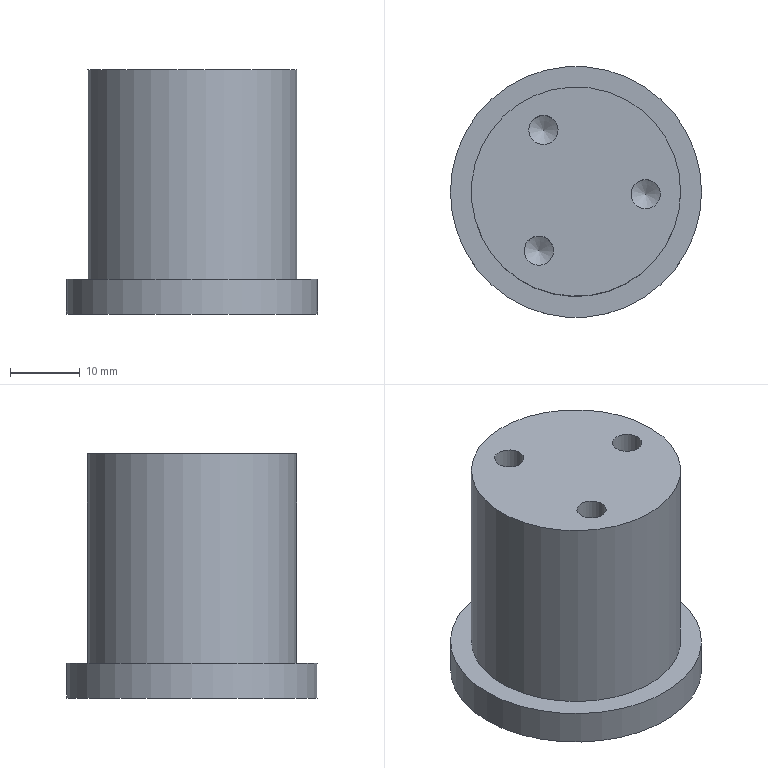Part | STEP file | 1 solid | 11 faces | box 36 x 36 x 35 mm | volume 25571 mm3 | cylinder 5 | plane 3 | cone 3 | commonest cylinder face diameters 4.2 x3 30 x1 36 x1
STEP:
#1=CARTESIAN_POINT('',(0.,0.,0.));
#2=DIRECTION('',(0.,0.,1.));
#3=DIRECTION('',(1.,0.,0.));
#4=AXIS2_PLACEMENT_3D('',#1,#2,#3);
#5=CARTESIAN_POINT('',(15.,0.,35.));
#6=VERTEX_POINT('',#5);
#7=CARTESIAN_POINT('',(0.,0.,35.));
#8=DIRECTION('',(0.,0.,-1.));
#9=DIRECTION('',(1.,0.,0.));
#10=AXIS2_PLACEMENT_3D('',#7,#8,#9);
#11=CIRCLE('',#10,15.);
#12=CARTESIAN_POINT('',(0.,0.,5.));
#13=DIRECTION('',(0.,0.,1.));
#14=DIRECTION('',(1.,0.,0.));
#15=AXIS2_PLACEMENT_3D('',#12,#13,#14);
#16=CYLINDRICAL_SURFACE('',#15,15.);
#17=CARTESIAN_POINT('',(6.283,30.));
#18=DIRECTION('',(-1.,0.));
#19=VECTOR('',#18,1.);
#20=LINE('',#17,#19);
#21=(GEOMETRIC_REPRESENTATION_CONTEXT(2)PARAMETRIC_REPRESENTATION_CONTEXT()REPRESENTATION_CONTEXT('',''));
#22=DEFINITIONAL_REPRESENTATION('',(#20),#21);
#23=PCURVE('',#16,#22);
#24=CARTESIAN_POINT('',(0.,0.,35.));
#25=DIRECTION('',(0.,0.,1.));
#26=DIRECTION('',(1.,0.,0.));
#27=AXIS2_PLACEMENT_3D('',#24,#25,#26);
#28=PLANE('',#27);
#29=CARTESIAN_POINT('',(15.,0.));
#30=CARTESIAN_POINT('',(15.,-25.981));
#31=CARTESIAN_POINT('',(-7.5,-12.99));
#32=CARTESIAN_POINT('',(-30.,0.));
#33=CARTESIAN_POINT('',(-7.5,12.99));
#34=CARTESIAN_POINT('',(15.,25.981));
#35=CARTESIAN_POINT('',(15.,0.));
#36=(BOUNDED_CURVE()B_SPLINE_CURVE(2,(#29,#30,#31,#32,#33,#34,#35),.UNSPECIFIED.,.T.,.F.)B_SPLINE_CURVE_WITH_KNOTS((1,2,2,2,2,1),(-2.094,0.,2.094,4.189,6.283,8.378),.UNSPECIFIED.)CURVE()GEOMETRIC_REPRESENTATION_ITEM()RATIONAL_B_SPLINE_CURVE((1.,0.5,1.,0.5,1.,0.5,1.))REPRESENTATION_ITEM(''));
#37=(GEOMETRIC_REPRESENTATION_CONTEXT(2)PARAMETRIC_REPRESENTATION_CONTEXT()REPRESENTATION_CONTEXT('',''));
#38=DEFINITIONAL_REPRESENTATION('',(#36),#37);
#39=PCURVE('',#28,#38);
#40=SURFACE_CURVE('',#11,(#23,#39),.PCURVE_S1.);
#41=EDGE_CURVE('',#6,#6,#40,.T.);
#42=ORIENTED_EDGE('',*,*,#41,.T.);
#43=CARTESIAN_POINT('',(15.,0.,5.));
#44=VERTEX_POINT('',#43);
#45=CARTESIAN_POINT('',(15.,0.,5.));
#46=CARTESIAN_POINT('',(15.,0.,35.));
#47=B_SPLINE_CURVE_WITH_KNOTS('',1,(#45,#46),.UNSPECIFIED.,.F.,.F.,(2,2),(0.,30.),.PIECEWISE_BEZIER_KNOTS.);
#48=CARTESIAN_POINT('',(0.,0.));
#49=DIRECTION('',(0.,1.));
#50=VECTOR('',#49,1.);
#51=LINE('',#48,#50);
#52=(GEOMETRIC_REPRESENTATION_CONTEXT(2)PARAMETRIC_REPRESENTATION_CONTEXT()REPRESENTATION_CONTEXT('',''));
#53=DEFINITIONAL_REPRESENTATION('',(#51),#52);
#54=PCURVE('',#16,#53);
#55=CARTESIAN_POINT('',(6.283,0.));
#56=DIRECTION('',(0.,1.));
#57=VECTOR('',#56,1.);
#58=LINE('',#55,#57);
#59=(GEOMETRIC_REPRESENTATION_CONTEXT(2)PARAMETRIC_REPRESENTATION_CONTEXT()REPRESENTATION_CONTEXT('',''));
#60=DEFINITIONAL_REPRESENTATION('',(#58),#59);
#61=PCURVE('',#16,#60);
#62=SEAM_CURVE('',#47,(#54,#61),.PCURVE_S1.);
#63=EDGE_CURVE('',#44,#6,#62,.T.);
#64=ORIENTED_EDGE('',*,*,#63,.F.);
#65=CARTESIAN_POINT('',(0.,0.,5.));
#66=DIRECTION('',(0.,0.,1.));
#67=DIRECTION('',(1.,0.,0.));
#68=AXIS2_PLACEMENT_3D('',#65,#66,#67);
#69=CIRCLE('',#68,15.);
#70=CARTESIAN_POINT('',(0.,0.));
#71=DIRECTION('',(1.,0.));
#72=VECTOR('',#71,1.);
#73=LINE('',#70,#72);
#74=(GEOMETRIC_REPRESENTATION_CONTEXT(2)PARAMETRIC_REPRESENTATION_CONTEXT()REPRESENTATION_CONTEXT('',''));
#75=DEFINITIONAL_REPRESENTATION('',(#73),#74);
#76=PCURVE('',#16,#75);
#77=CARTESIAN_POINT('',(0.,0.,5.));
#78=DIRECTION('',(0.,0.,1.));
#79=DIRECTION('',(1.,0.,0.));
#80=AXIS2_PLACEMENT_3D('',#77,#78,#79);
#81=PLANE('',#80);
#82=CARTESIAN_POINT('',(0.,0.));
#83=DIRECTION('',(1.,0.));
#84=AXIS2_PLACEMENT_2D('',#82,#83);
#85=CIRCLE('',#84,15.);
#86=(GEOMETRIC_REPRESENTATION_CONTEXT(2)PARAMETRIC_REPRESENTATION_CONTEXT()REPRESENTATION_CONTEXT('',''));
#87=DEFINITIONAL_REPRESENTATION('',(#85),#86);
#88=PCURVE('',#81,#87);
#89=SURFACE_CURVE('',#69,(#76,#88),.PCURVE_S1.);
#90=EDGE_CURVE('',#44,#44,#89,.T.);
#91=ORIENTED_EDGE('',*,*,#90,.T.);
#92=ORIENTED_EDGE('',*,*,#63,.T.);
#93=EDGE_LOOP('',(#42,#64,#91,#92));
#94=FACE_BOUND('',#93,.T.);
#95=ADVANCED_FACE('',(#94),#16,.T.);
#96=CARTESIAN_POINT('',(-2.577,8.839,35.));
#97=VERTEX_POINT('',#96);
#98=CARTESIAN_POINT('',(-4.677,8.839,35.));
#99=DIRECTION('',(0.,0.,-1.));
#100=DIRECTION('',(1.,0.,0.));
#101=AXIS2_PLACEMENT_3D('',#98,#99,#100);
#102=CIRCLE('',#101,2.1);
#103=CARTESIAN_POINT('',(-2.577,8.839));
#104=CARTESIAN_POINT('',(-2.577,5.201));
#105=CARTESIAN_POINT('',(-5.727,7.02));
#106=CARTESIAN_POINT('',(-8.877,8.839));
#107=CARTESIAN_POINT('',(-5.727,10.657));
#108=CARTESIAN_POINT('',(-2.577,12.476));
#109=CARTESIAN_POINT('',(-2.577,8.839));
#110=(BOUNDED_CURVE()B_SPLINE_CURVE(2,(#103,#104,#105,#106,#107,#108,#109),.UNSPECIFIED.,.T.,.F.)B_SPLINE_CURVE_WITH_KNOTS((1,2,2,2,2,1),(-2.094,0.,2.094,4.189,6.283,8.378),.UNSPECIFIED.)CURVE()GEOMETRIC_REPRESENTATION_ITEM()RATIONAL_B_SPLINE_CURVE((1.,0.5,1.,0.5,1.,0.5,1.))REPRESENTATION_ITEM(''));
#111=(GEOMETRIC_REPRESENTATION_CONTEXT(2)PARAMETRIC_REPRESENTATION_CONTEXT()REPRESENTATION_CONTEXT('',''));
#112=DEFINITIONAL_REPRESENTATION('',(#110),#111);
#113=PCURVE('',#28,#112);
#114=CARTESIAN_POINT('',(-4.677,8.839,35.));
#115=DIRECTION('',(0.,0.,1.));
#116=DIRECTION('',(1.,0.,0.));
#117=AXIS2_PLACEMENT_3D('',#114,#115,#116);
#118=CYLINDRICAL_SURFACE('',#117,2.1);
#119=CARTESIAN_POINT('',(6.283,0.));
#120=DIRECTION('',(-1.,0.));
#121=VECTOR('',#120,1.);
#122=LINE('',#119,#121);
#123=(GEOMETRIC_REPRESENTATION_CONTEXT(2)PARAMETRIC_REPRESENTATION_CONTEXT()REPRESENTATION_CONTEXT('',''));
#124=DEFINITIONAL_REPRESENTATION('',(#122),#123);
#125=PCURVE('',#118,#124);
#126=SURFACE_CURVE('',#102,(#113,#125),.PCURVE_S1.);
#127=EDGE_CURVE('',#97,#97,#126,.T.);
#128=ORIENTED_EDGE('',*,*,#127,.T.);
#129=EDGE_LOOP('',(#128));
#130=FACE_BOUND('',#129,.T.);
#131=CARTESIAN_POINT('',(-3.216,-8.47,35.));
#132=VERTEX_POINT('',#131);
#133=CARTESIAN_POINT('',(-5.316,-8.47,35.));
#134=DIRECTION('',(0.,0.,-1.));
#135=DIRECTION('',(1.,0.,0.));
#136=AXIS2_PLACEMENT_3D('',#133,#134,#135);
#137=CIRCLE('',#136,2.1);
#138=CARTESIAN_POINT('',(-3.216,-8.47));
#139=CARTESIAN_POINT('',(-3.216,-12.107));
#140=CARTESIAN_POINT('',(-6.366,-10.289));
#141=CARTESIAN_POINT('',(-9.516,-8.47));
#142=CARTESIAN_POINT('',(-6.366,-6.651));
#143=CARTESIAN_POINT('',(-3.216,-4.833));
#144=CARTESIAN_POINT('',(-3.216,-8.47));
#145=(BOUNDED_CURVE()B_SPLINE_CURVE(2,(#138,#139,#140,#141,#142,#143,#144),.UNSPECIFIED.,.T.,.F.)B_SPLINE_CURVE_WITH_KNOTS((1,2,2,2,2,1),(-2.094,0.,2.094,4.189,6.283,8.378),.UNSPECIFIED.)CURVE()GEOMETRIC_REPRESENTATION_ITEM()RATIONAL_B_SPLINE_CURVE((1.,0.5,1.,0.5,1.,0.5,1.))REPRESENTATION_ITEM(''));
#146=(GEOMETRIC_REPRESENTATION_CONTEXT(2)PARAMETRIC_REPRESENTATION_CONTEXT()REPRESENTATION_CONTEXT('',''));
#147=DEFINITIONAL_REPRESENTATION('',(#145),#146);
#148=PCURVE('',#28,#147);
#149=CARTESIAN_POINT('',(-5.316,-8.47,35.));
#150=DIRECTION('',(0.,0.,1.));
#151=DIRECTION('',(1.,0.,0.));
#152=AXIS2_PLACEMENT_3D('',#149,#150,#151);
#153=CYLINDRICAL_SURFACE('',#152,2.1);
#154=CARTESIAN_POINT('',(6.283,0.));
#155=DIRECTION('',(-1.,0.));
#156=VECTOR('',#155,1.);
#157=LINE('',#154,#156);
#158=(GEOMETRIC_REPRESENTATION_CONTEXT(2)PARAMETRIC_REPRESENTATION_CONTEXT()REPRESENTATION_CONTEXT('',''));
#159=DEFINITIONAL_REPRESENTATION('',(#157),#158);
#160=PCURVE('',#153,#159);
#161=SURFACE_CURVE('',#137,(#148,#160),.PCURVE_S1.);
#162=EDGE_CURVE('',#132,#132,#161,.T.);
#163=ORIENTED_EDGE('',*,*,#162,.T.);
#164=EDGE_LOOP('',(#163));
#165=FACE_BOUND('',#164,.T.);
#166=CARTESIAN_POINT('',(12.093,-0.3685,35.));
#167=VERTEX_POINT('',#166);
#168=CARTESIAN_POINT('',(9.993,-0.3685,35.));
#169=DIRECTION('',(0.,0.,-1.));
#170=DIRECTION('',(1.,0.,0.));
#171=AXIS2_PLACEMENT_3D('',#168,#169,#170);
#172=CIRCLE('',#171,2.1);
#173=CARTESIAN_POINT('',(12.093,-0.3685));
#174=CARTESIAN_POINT('',(12.093,-4.006));
#175=CARTESIAN_POINT('',(8.943,-2.187));
#176=CARTESIAN_POINT('',(5.793,-0.3685));
#177=CARTESIAN_POINT('',(8.943,1.45));
#178=CARTESIAN_POINT('',(12.093,3.269));
#179=CARTESIAN_POINT('',(12.093,-0.3685));
#180=(BOUNDED_CURVE()B_SPLINE_CURVE(2,(#173,#174,#175,#176,#177,#178,#179),.UNSPECIFIED.,.T.,.F.)B_SPLINE_CURVE_WITH_KNOTS((1,2,2,2,2,1),(-2.094,0.,2.094,4.189,6.283,8.378),.UNSPECIFIED.)CURVE()GEOMETRIC_REPRESENTATION_ITEM()RATIONAL_B_SPLINE_CURVE((1.,0.5,1.,0.5,1.,0.5,1.))REPRESENTATION_ITEM(''));
#181=(GEOMETRIC_REPRESENTATION_CONTEXT(2)PARAMETRIC_REPRESENTATION_CONTEXT()REPRESENTATION_CONTEXT('',''));
#182=DEFINITIONAL_REPRESENTATION('',(#180),#181);
#183=PCURVE('',#28,#182);
#184=CARTESIAN_POINT('',(9.993,-0.3685,35.));
#185=DIRECTION('',(0.,0.,1.));
#186=DIRECTION('',(1.,0.,0.));
#187=AXIS2_PLACEMENT_3D('',#184,#185,#186);
#188=CYLINDRICAL_SURFACE('',#187,2.1);
#189=CARTESIAN_POINT('',(6.283,0.));
#190=DIRECTION('',(-1.,0.));
#191=VECTOR('',#190,1.);
#192=LINE('',#189,#191);
#193=(GEOMETRIC_REPRESENTATION_CONTEXT(2)PARAMETRIC_REPRESENTATION_CONTEXT()REPRESENTATION_CONTEXT('',''));
#194=DEFINITIONAL_REPRESENTATION('',(#192),#193);
#195=PCURVE('',#188,#194);
#196=SURFACE_CURVE('',#172,(#183,#195),.PCURVE_S1.);
#197=EDGE_CURVE('',#167,#167,#196,.T.);
#198=ORIENTED_EDGE('',*,*,#197,.T.);
#199=EDGE_LOOP('',(#198));
#200=FACE_BOUND('',#199,.T.);
#201=ORIENTED_EDGE('',*,*,#41,.F.);
#202=EDGE_LOOP('',(#201));
#203=FACE_BOUND('',#202,.T.);
#204=ADVANCED_FACE('',(#130,#165,#200,#203),#28,.T.);
#205=ORIENTED_EDGE('',*,*,#90,.F.);
#206=EDGE_LOOP('',(#205));
#207=FACE_BOUND('',#206,.T.);
#208=CARTESIAN_POINT('',(-18.,0.,5.));
#209=VERTEX_POINT('',#208);
#210=CARTESIAN_POINT('',(0.,0.,5.));
#211=DIRECTION('',(0.,0.,1.));
#212=DIRECTION('',(-1.,0.,0.));
#213=AXIS2_PLACEMENT_3D('',#210,#211,#212);
#214=CIRCLE('',#213,18.);
#215=CARTESIAN_POINT('',(0.,0.));
#216=DIRECTION('',(-1.,0.));
#217=AXIS2_PLACEMENT_2D('',#215,#216);
#218=CIRCLE('',#217,18.);
#219=(GEOMETRIC_REPRESENTATION_CONTEXT(2)PARAMETRIC_REPRESENTATION_CONTEXT()REPRESENTATION_CONTEXT('',''));
#220=DEFINITIONAL_REPRESENTATION('',(#218),#219);
#221=PCURVE('',#81,#220);
#222=CARTESIAN_POINT('',(0.,0.,35.));
#223=DIRECTION('',(0.,0.,-1.));
#224=DIRECTION('',(-1.,0.,0.));
#225=AXIS2_PLACEMENT_3D('',#222,#223,#224);
#226=CYLINDRICAL_SURFACE('',#225,18.);
#227=CARTESIAN_POINT('',(6.283,30.));
#228=DIRECTION('',(-1.,0.));
#229=VECTOR('',#228,1.);
#230=LINE('',#227,#229);
#231=(GEOMETRIC_REPRESENTATION_CONTEXT(2)PARAMETRIC_REPRESENTATION_CONTEXT()REPRESENTATION_CONTEXT('',''));
#232=DEFINITIONAL_REPRESENTATION('',(#230),#231);
#233=PCURVE('',#226,#232);
#234=SURFACE_CURVE('',#214,(#221,#233),.PCURVE_S1.);
#235=EDGE_CURVE('',#209,#209,#234,.T.);
#236=ORIENTED_EDGE('',*,*,#235,.T.);
#237=EDGE_LOOP('',(#236));
#238=FACE_BOUND('',#237,.T.);
#239=ADVANCED_FACE('',(#207,#238),#81,.T.);
#240=ORIENTED_EDGE('',*,*,#127,.T.);
#241=CARTESIAN_POINT('',(-2.577,8.839,18.));
#242=VERTEX_POINT('',#241);
#243=CARTESIAN_POINT('',(-2.577,8.839,18.));
#244=CARTESIAN_POINT('',(-2.577,8.839,35.));
#245=B_SPLINE_CURVE_WITH_KNOTS('',1,(#243,#244),.UNSPECIFIED.,.F.,.F.,(2,2),(-17.,0.),.PIECEWISE_BEZIER_KNOTS.);
#246=CARTESIAN_POINT('',(0.,0.));
#247=DIRECTION('',(0.,1.));
#248=VECTOR('',#247,1.);
#249=LINE('',#246,#248);
#250=(GEOMETRIC_REPRESENTATION_CONTEXT(2)PARAMETRIC_REPRESENTATION_CONTEXT()REPRESENTATION_CONTEXT('',''));
#251=DEFINITIONAL_REPRESENTATION('',(#249),#250);
#252=PCURVE('',#118,#251);
#253=CARTESIAN_POINT('',(6.283,0.));
#254=DIRECTION('',(0.,1.));
#255=VECTOR('',#254,1.);
#256=LINE('',#253,#255);
#257=(GEOMETRIC_REPRESENTATION_CONTEXT(2)PARAMETRIC_REPRESENTATION_CONTEXT()REPRESENTATION_CONTEXT('',''));
#258=DEFINITIONAL_REPRESENTATION('',(#256),#257);
#259=PCURVE('',#118,#258);
#260=SEAM_CURVE('',#245,(#252,#259),.PCURVE_S1.);
#261=EDGE_CURVE('',#242,#97,#260,.T.);
#262=ORIENTED_EDGE('',*,*,#261,.F.);
#263=CARTESIAN_POINT('',(-4.677,8.839,18.));
#264=DIRECTION('',(0.,0.,1.));
#265=DIRECTION('',(1.,0.,0.));
#266=AXIS2_PLACEMENT_3D('',#263,#264,#265);
#267=CIRCLE('',#266,2.1);
#268=CARTESIAN_POINT('',(0.,-17.));
#269=DIRECTION('',(1.,0.));
#270=VECTOR('',#269,1.);
#271=LINE('',#268,#270);
#272=(GEOMETRIC_REPRESENTATION_CONTEXT(2)PARAMETRIC_REPRESENTATION_CONTEXT()REPRESENTATION_CONTEXT('',''));
#273=DEFINITIONAL_REPRESENTATION('',(#271),#272);
#274=PCURVE('',#118,#273);
#275=CARTESIAN_POINT('',(-4.677,8.839,18.));
#276=DIRECTION('',(0.,0.,1.));
#277=DIRECTION('',(1.,0.,0.));
#278=AXIS2_PLACEMENT_3D('',#275,#276,#277);
#279=CONICAL_SURFACE('',#278,2.1,1.03);
#280=CARTESIAN_POINT('',(0.,0.));
#281=DIRECTION('',(1.,0.));
#282=VECTOR('',#281,1.);
#283=LINE('',#280,#282);
#284=(GEOMETRIC_REPRESENTATION_CONTEXT(2)PARAMETRIC_REPRESENTATION_CONTEXT()REPRESENTATION_CONTEXT('',''));
#285=DEFINITIONAL_REPRESENTATION('',(#283),#284);
#286=PCURVE('',#279,#285);
#287=SURFACE_CURVE('',#267,(#274,#286),.PCURVE_S1.);
#288=EDGE_CURVE('',#242,#242,#287,.T.);
#289=ORIENTED_EDGE('',*,*,#288,.T.);
#290=ORIENTED_EDGE('',*,*,#261,.T.);
#291=EDGE_LOOP('',(#240,#262,#289,#290));
#292=FACE_BOUND('',#291,.F.);
#293=ADVANCED_FACE('',(#292),#118,.F.);
#294=ORIENTED_EDGE('',*,*,#162,.T.);
#295=CARTESIAN_POINT('',(-3.216,-8.47,18.));
#296=VERTEX_POINT('',#295);
#297=CARTESIAN_POINT('',(-3.216,-8.47,18.));
#298=CARTESIAN_POINT('',(-3.216,-8.47,35.));
#299=B_SPLINE_CURVE_WITH_KNOTS('',1,(#297,#298),.UNSPECIFIED.,.F.,.F.,(2,2),(-17.,0.),.PIECEWISE_BEZIER_KNOTS.);
#300=CARTESIAN_POINT('',(0.,0.));
#301=DIRECTION('',(0.,1.));
#302=VECTOR('',#301,1.);
#303=LINE('',#300,#302);
#304=(GEOMETRIC_REPRESENTATION_CONTEXT(2)PARAMETRIC_REPRESENTATION_CONTEXT()REPRESENTATION_CONTEXT('',''));
#305=DEFINITIONAL_REPRESENTATION('',(#303),#304);
#306=PCURVE('',#153,#305);
#307=CARTESIAN_POINT('',(6.283,0.));
#308=DIRECTION('',(0.,1.));
#309=VECTOR('',#308,1.);
#310=LINE('',#307,#309);
#311=(GEOMETRIC_REPRESENTATION_CONTEXT(2)PARAMETRIC_REPRESENTATION_CONTEXT()REPRESENTATION_CONTEXT('',''));
#312=DEFINITIONAL_REPRESENTATION('',(#310),#311);
#313=PCURVE('',#153,#312);
#314=SEAM_CURVE('',#299,(#306,#313),.PCURVE_S1.);
#315=EDGE_CURVE('',#296,#132,#314,.T.);
#316=ORIENTED_EDGE('',*,*,#315,.F.);
#317=CARTESIAN_POINT('',(-5.316,-8.47,18.));
#318=DIRECTION('',(0.,0.,1.));
#319=DIRECTION('',(1.,0.,0.));
#320=AXIS2_PLACEMENT_3D('',#317,#318,#319);
#321=CIRCLE('',#320,2.1);
#322=CARTESIAN_POINT('',(0.,-17.));
#323=DIRECTION('',(1.,0.));
#324=VECTOR('',#323,1.);
#325=LINE('',#322,#324);
#326=(GEOMETRIC_REPRESENTATION_CONTEXT(2)PARAMETRIC_REPRESENTATION_CONTEXT()REPRESENTATION_CONTEXT('',''));
#327=DEFINITIONAL_REPRESENTATION('',(#325),#326);
#328=PCURVE('',#153,#327);
#329=CARTESIAN_POINT('',(-5.316,-8.47,18.));
#330=DIRECTION('',(0.,0.,1.));
#331=DIRECTION('',(1.,0.,0.));
#332=AXIS2_PLACEMENT_3D('',#329,#330,#331);
#333=CONICAL_SURFACE('',#332,2.1,1.03);
#334=CARTESIAN_POINT('',(0.,0.));
#335=DIRECTION('',(1.,0.));
#336=VECTOR('',#335,1.);
#337=LINE('',#334,#336);
#338=(GEOMETRIC_REPRESENTATION_CONTEXT(2)PARAMETRIC_REPRESENTATION_CONTEXT()REPRESENTATION_CONTEXT('',''));
#339=DEFINITIONAL_REPRESENTATION('',(#337),#338);
#340=PCURVE('',#333,#339);
#341=SURFACE_CURVE('',#321,(#328,#340),.PCURVE_S1.);
#342=EDGE_CURVE('',#296,#296,#341,.T.);
#343=ORIENTED_EDGE('',*,*,#342,.T.);
#344=ORIENTED_EDGE('',*,*,#315,.T.);
#345=EDGE_LOOP('',(#294,#316,#343,#344));
#346=FACE_BOUND('',#345,.F.);
#347=ADVANCED_FACE('',(#346),#153,.F.);
#348=ORIENTED_EDGE('',*,*,#197,.T.);
#349=CARTESIAN_POINT('',(12.093,-0.3685,18.));
#350=VERTEX_POINT('',#349);
#351=CARTESIAN_POINT('',(12.093,-0.3685,18.));
#352=CARTESIAN_POINT('',(12.093,-0.3685,35.));
#353=B_SPLINE_CURVE_WITH_KNOTS('',1,(#351,#352),.UNSPECIFIED.,.F.,.F.,(2,2),(-17.,0.),.PIECEWISE_BEZIER_KNOTS.);
#354=CARTESIAN_POINT('',(0.,0.));
#355=DIRECTION('',(0.,1.));
#356=VECTOR('',#355,1.);
#357=LINE('',#354,#356);
#358=(GEOMETRIC_REPRESENTATION_CONTEXT(2)PARAMETRIC_REPRESENTATION_CONTEXT()REPRESENTATION_CONTEXT('',''));
#359=DEFINITIONAL_REPRESENTATION('',(#357),#358);
#360=PCURVE('',#188,#359);
#361=CARTESIAN_POINT('',(6.283,0.));
#362=DIRECTION('',(0.,1.));
#363=VECTOR('',#362,1.);
#364=LINE('',#361,#363);
#365=(GEOMETRIC_REPRESENTATION_CONTEXT(2)PARAMETRIC_REPRESENTATION_CONTEXT()REPRESENTATION_CONTEXT('',''));
#366=DEFINITIONAL_REPRESENTATION('',(#364),#365);
#367=PCURVE('',#188,#366);
#368=SEAM_CURVE('',#353,(#360,#367),.PCURVE_S1.);
#369=EDGE_CURVE('',#350,#167,#368,.T.);
#370=ORIENTED_EDGE('',*,*,#369,.F.);
#371=CARTESIAN_POINT('',(9.993,-0.3685,18.));
#372=DIRECTION('',(0.,0.,1.));
#373=DIRECTION('',(1.,0.,0.));
#374=AXIS2_PLACEMENT_3D('',#371,#372,#373);
#375=CIRCLE('',#374,2.1);
#376=CARTESIAN_POINT('',(0.,-17.));
#377=DIRECTION('',(1.,0.));
#378=VECTOR('',#377,1.);
#379=LINE('',#376,#378);
#380=(GEOMETRIC_REPRESENTATION_CONTEXT(2)PARAMETRIC_REPRESENTATION_CONTEXT()REPRESENTATION_CONTEXT('',''));
#381=DEFINITIONAL_REPRESENTATION('',(#379),#380);
#382=PCURVE('',#188,#381);
#383=CARTESIAN_POINT('',(9.993,-0.3685,18.));
#384=DIRECTION('',(0.,0.,1.));
#385=DIRECTION('',(1.,0.,0.));
#386=AXIS2_PLACEMENT_3D('',#383,#384,#385);
#387=CONICAL_SURFACE('',#386,2.1,1.03);
#388=CARTESIAN_POINT('',(0.,0.));
#389=DIRECTION('',(1.,0.));
#390=VECTOR('',#389,1.);
#391=LINE('',#388,#390);
#392=(GEOMETRIC_REPRESENTATION_CONTEXT(2)PARAMETRIC_REPRESENTATION_CONTEXT()REPRESENTATION_CONTEXT('',''));
#393=DEFINITIONAL_REPRESENTATION('',(#391),#392);
#394=PCURVE('',#387,#393);
#395=SURFACE_CURVE('',#375,(#382,#394),.PCURVE_S1.);
#396=EDGE_CURVE('',#350,#350,#395,.T.);
#397=ORIENTED_EDGE('',*,*,#396,.T.);
#398=ORIENTED_EDGE('',*,*,#369,.T.);
#399=EDGE_LOOP('',(#348,#370,#397,#398));
#400=FACE_BOUND('',#399,.F.);
#401=ADVANCED_FACE('',(#400),#188,.F.);
#402=CARTESIAN_POINT('',(-18.,0.,0.));
#403=VERTEX_POINT('',#402);
#404=CARTESIAN_POINT('',(0.,0.,0.));
#405=DIRECTION('',(0.,0.,1.));
#406=DIRECTION('',(-1.,0.,0.));
#407=AXIS2_PLACEMENT_3D('',#404,#405,#406);
#408=CIRCLE('',#407,18.);
#409=CARTESIAN_POINT('',(6.283,35.));
#410=DIRECTION('',(-1.,0.));
#411=VECTOR('',#410,1.);
#412=LINE('',#409,#411);
#413=(GEOMETRIC_REPRESENTATION_CONTEXT(2)PARAMETRIC_REPRESENTATION_CONTEXT()REPRESENTATION_CONTEXT('',''));
#414=DEFINITIONAL_REPRESENTATION('',(#412),#413);
#415=PCURVE('',#226,#414);
#416=CARTESIAN_POINT('',(0.,0.,0.));
#417=DIRECTION('',(0.,0.,1.));
#418=DIRECTION('',(1.,0.,0.));
#419=AXIS2_PLACEMENT_3D('',#416,#417,#418);
#420=PLANE('',#419);
#421=CARTESIAN_POINT('',(0.,0.));
#422=DIRECTION('',(-1.,0.));
#423=AXIS2_PLACEMENT_2D('',#421,#422);
#424=CIRCLE('',#423,18.);
#425=(GEOMETRIC_REPRESENTATION_CONTEXT(2)PARAMETRIC_REPRESENTATION_CONTEXT()REPRESENTATION_CONTEXT('',''));
#426=DEFINITIONAL_REPRESENTATION('',(#424),#425);
#427=PCURVE('',#420,#426);
#428=SURFACE_CURVE('',#408,(#415,#427),.PCURVE_S1.);
#429=EDGE_CURVE('',#403,#403,#428,.T.);
#430=ORIENTED_EDGE('',*,*,#429,.T.);
#431=CARTESIAN_POINT('',(-18.,0.,5.));
#432=CARTESIAN_POINT('',(-18.,0.,0.));
#433=B_SPLINE_CURVE_WITH_KNOTS('',1,(#431,#432),.UNSPECIFIED.,.F.,.F.,(2,2),(30.,35.),.PIECEWISE_BEZIER_KNOTS.);
#434=CARTESIAN_POINT('',(0.,0.));
#435=DIRECTION('',(0.,1.));
#436=VECTOR('',#435,1.);
#437=LINE('',#434,#436);
#438=(GEOMETRIC_REPRESENTATION_CONTEXT(2)PARAMETRIC_REPRESENTATION_CONTEXT()REPRESENTATION_CONTEXT('',''));
#439=DEFINITIONAL_REPRESENTATION('',(#437),#438);
#440=PCURVE('',#226,#439);
#441=CARTESIAN_POINT('',(6.283,0.));
#442=DIRECTION('',(0.,1.));
#443=VECTOR('',#442,1.);
#444=LINE('',#441,#443);
#445=(GEOMETRIC_REPRESENTATION_CONTEXT(2)PARAMETRIC_REPRESENTATION_CONTEXT()REPRESENTATION_CONTEXT('',''));
#446=DEFINITIONAL_REPRESENTATION('',(#444),#445);
#447=PCURVE('',#226,#446);
#448=SEAM_CURVE('',#433,(#440,#447),.PCURVE_S1.);
#449=EDGE_CURVE('',#209,#403,#448,.T.);
#450=ORIENTED_EDGE('',*,*,#449,.F.);
#451=ORIENTED_EDGE('',*,*,#235,.F.);
#452=ORIENTED_EDGE('',*,*,#449,.T.);
#453=EDGE_LOOP('',(#430,#450,#451,#452));
#454=FACE_BOUND('',#453,.T.);
#455=ADVANCED_FACE('',(#454),#226,.T.);
#456=ORIENTED_EDGE('',*,*,#288,.F.);
#457=CARTESIAN_POINT('',(-4.677,8.839,16.738));
#458=VERTEX_POINT('',#457);
#459=CARTESIAN_POINT('',(-4.677,8.839,16.738));
#460=CARTESIAN_POINT('',(-2.577,8.839,18.));
#461=B_SPLINE_CURVE_WITH_KNOTS('',1,(#459,#460),.UNSPECIFIED.,.F.,.F.,(2,2),(-2.45,0.),.PIECEWISE_BEZIER_KNOTS.);
#462=CARTESIAN_POINT('',(0.,0.));
#463=DIRECTION('',(0.,1.));
#464=VECTOR('',#463,1.);
#465=LINE('',#462,#464);
#466=(GEOMETRIC_REPRESENTATION_CONTEXT(2)PARAMETRIC_REPRESENTATION_CONTEXT()REPRESENTATION_CONTEXT('',''));
#467=DEFINITIONAL_REPRESENTATION('',(#465),#466);
#468=PCURVE('',#279,#467);
#469=CARTESIAN_POINT('',(6.283,0.));
#470=DIRECTION('',(0.,1.));
#471=VECTOR('',#470,1.);
#472=LINE('',#469,#471);
#473=(GEOMETRIC_REPRESENTATION_CONTEXT(2)PARAMETRIC_REPRESENTATION_CONTEXT()REPRESENTATION_CONTEXT('',''));
#474=DEFINITIONAL_REPRESENTATION('',(#472),#473);
#475=PCURVE('',#279,#474);
#476=SEAM_CURVE('',#461,(#468,#475),.PCURVE_S1.);
#477=EDGE_CURVE('',#458,#242,#476,.T.);
#478=ORIENTED_EDGE('',*,*,#477,.F.);
#479=ORIENTED_EDGE('',*,*,#477,.T.);
#480=EDGE_LOOP('',(#456,#478,#479));
#481=FACE_BOUND('',#480,.F.);
#482=ADVANCED_FACE('',(#481),#279,.F.);
#483=ORIENTED_EDGE('',*,*,#342,.F.);
#484=CARTESIAN_POINT('',(-5.316,-8.47,16.738));
#485=VERTEX_POINT('',#484);
#486=CARTESIAN_POINT('',(-5.316,-8.47,16.738));
#487=CARTESIAN_POINT('',(-3.216,-8.47,18.));
#488=B_SPLINE_CURVE_WITH_KNOTS('',1,(#486,#487),.UNSPECIFIED.,.F.,.F.,(2,2),(-2.45,0.),.PIECEWISE_BEZIER_KNOTS.);
#489=CARTESIAN_POINT('',(0.,0.));
#490=DIRECTION('',(0.,1.));
#491=VECTOR('',#490,1.);
#492=LINE('',#489,#491);
#493=(GEOMETRIC_REPRESENTATION_CONTEXT(2)PARAMETRIC_REPRESENTATION_CONTEXT()REPRESENTATION_CONTEXT('',''));
#494=DEFINITIONAL_REPRESENTATION('',(#492),#493);
#495=PCURVE('',#333,#494);
#496=CARTESIAN_POINT('',(6.283,0.));
#497=DIRECTION('',(0.,1.));
#498=VECTOR('',#497,1.);
#499=LINE('',#496,#498);
#500=(GEOMETRIC_REPRESENTATION_CONTEXT(2)PARAMETRIC_REPRESENTATION_CONTEXT()REPRESENTATION_CONTEXT('',''));
#501=DEFINITIONAL_REPRESENTATION('',(#499),#500);
#502=PCURVE('',#333,#501);
#503=SEAM_CURVE('',#488,(#495,#502),.PCURVE_S1.);
#504=EDGE_CURVE('',#485,#296,#503,.T.);
#505=ORIENTED_EDGE('',*,*,#504,.F.);
#506=ORIENTED_EDGE('',*,*,#504,.T.);
#507=EDGE_LOOP('',(#483,#505,#506));
#508=FACE_BOUND('',#507,.F.);
#509=ADVANCED_FACE('',(#508),#333,.F.);
#510=ORIENTED_EDGE('',*,*,#396,.F.);
#511=CARTESIAN_POINT('',(9.993,-0.3685,16.738));
#512=VERTEX_POINT('',#511);
#513=CARTESIAN_POINT('',(9.993,-0.3685,16.738));
#514=CARTESIAN_POINT('',(12.093,-0.3685,18.));
#515=B_SPLINE_CURVE_WITH_KNOTS('',1,(#513,#514),.UNSPECIFIED.,.F.,.F.,(2,2),(-2.45,0.),.PIECEWISE_BEZIER_KNOTS.);
#516=CARTESIAN_POINT('',(0.,0.));
#517=DIRECTION('',(0.,1.));
#518=VECTOR('',#517,1.);
#519=LINE('',#516,#518);
#520=(GEOMETRIC_REPRESENTATION_CONTEXT(2)PARAMETRIC_REPRESENTATION_CONTEXT()REPRESENTATION_CONTEXT('',''));
#521=DEFINITIONAL_REPRESENTATION('',(#519),#520);
#522=PCURVE('',#387,#521);
#523=CARTESIAN_POINT('',(6.283,0.));
#524=DIRECTION('',(0.,1.));
#525=VECTOR('',#524,1.);
#526=LINE('',#523,#525);
#527=(GEOMETRIC_REPRESENTATION_CONTEXT(2)PARAMETRIC_REPRESENTATION_CONTEXT()REPRESENTATION_CONTEXT('',''));
#528=DEFINITIONAL_REPRESENTATION('',(#526),#527);
#529=PCURVE('',#387,#528);
#530=SEAM_CURVE('',#515,(#522,#529),.PCURVE_S1.);
#531=EDGE_CURVE('',#512,#350,#530,.T.);
#532=ORIENTED_EDGE('',*,*,#531,.F.);
#533=ORIENTED_EDGE('',*,*,#531,.T.);
#534=EDGE_LOOP('',(#510,#532,#533));
#535=FACE_BOUND('',#534,.F.);
#536=ADVANCED_FACE('',(#535),#387,.F.);
#537=ORIENTED_EDGE('',*,*,#429,.F.);
#538=EDGE_LOOP('',(#537));
#539=FACE_BOUND('',#538,.T.);
#540=ADVANCED_FACE('',(#539),#420,.F.);
#541=CLOSED_SHELL('',(#95,#204,#239,#293,#347,#401,#455,#482,#509,#536,#540));
#542=MANIFOLD_SOLID_BREP('',#541);
#543=(LENGTH_UNIT()NAMED_UNIT(*)SI_UNIT(.MILLI.,.METRE.));
#544=UNCERTAINTY_MEASURE_WITH_UNIT(LENGTH_MEASURE(0.00001),#543,'','');
#545=(NAMED_UNIT(*)PLANE_ANGLE_UNIT()SI_UNIT($,.RADIAN.));
#546=(NAMED_UNIT(*)SI_UNIT($,.STERADIAN.)SOLID_ANGLE_UNIT());
#547=(GEOMETRIC_REPRESENTATION_CONTEXT(3)GLOBAL_UNCERTAINTY_ASSIGNED_CONTEXT((#544))GLOBAL_UNIT_ASSIGNED_CONTEXT((#543,#545,#546))REPRESENTATION_CONTEXT('',''));
#548=ADVANCED_BREP_SHAPE_REPRESENTATION('',(#4,#542),#547);